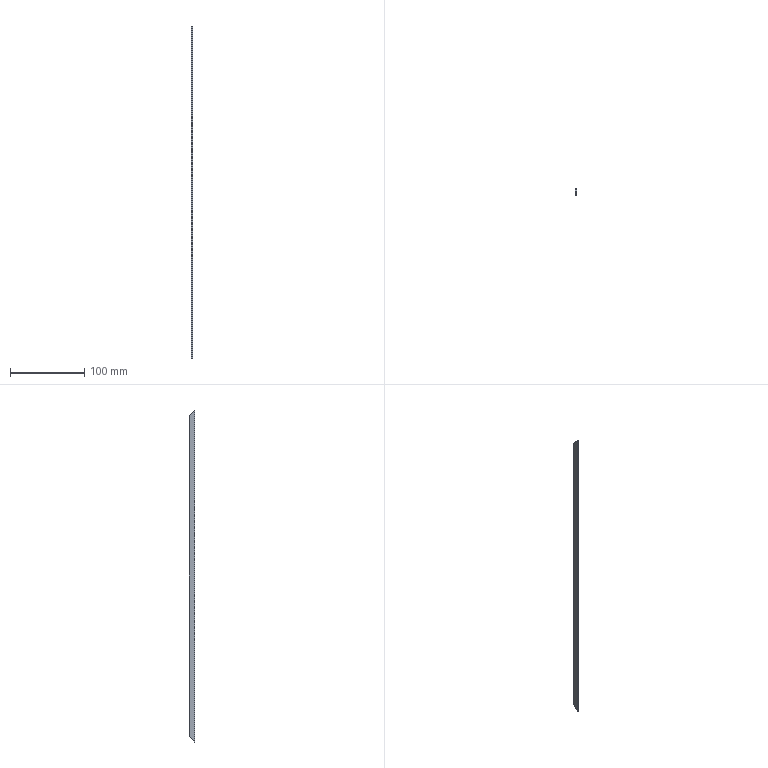Part | NX | features BREP 1 | 1 solid | 6 faces | box 1.5 x 8 x 447.9 mm | volume 5279 mm3 | plane 6
STEP:
#1=CARTESIAN_POINT('',(0.,8.,215.95));
#2=VERTEX_POINT('',#1);
#3=CARTESIAN_POINT('',(0.,8.,-215.95));
#4=VERTEX_POINT('',#3);
#5=CARTESIAN_POINT('',(0.,8.,223.95));
#6=DIRECTION('',(0.,0.,-1.));
#7=VECTOR('',#6,1000.);
#8=LINE('',#5,#7);
#9=EDGE_CURVE('',#2,#4,#8,.T.);
#10=ORIENTED_EDGE('',*,*,#9,.T.);
#11=CARTESIAN_POINT('',(0.,0.,-223.95));
#12=VERTEX_POINT('',#11);
#13=CARTESIAN_POINT('',(0.,8.,-215.95));
#14=DIRECTION('',(0.,-0.7071,-0.7071));
#15=VECTOR('',#14,1000.);
#16=LINE('',#13,#15);
#17=EDGE_CURVE('',#4,#12,#16,.T.);
#18=ORIENTED_EDGE('',*,*,#17,.T.);
#19=CARTESIAN_POINT('',(0.,0.,223.95));
#20=VERTEX_POINT('',#19);
#21=CARTESIAN_POINT('',(0.,0.,223.95));
#22=DIRECTION('',(0.,0.,-1.));
#23=VECTOR('',#22,1000.);
#24=LINE('',#21,#23);
#25=EDGE_CURVE('',#20,#12,#24,.T.);
#26=ORIENTED_EDGE('',*,*,#25,.F.);
#27=CARTESIAN_POINT('',(0.,0.,223.95));
#28=DIRECTION('',(0.,0.7071,-0.7071));
#29=VECTOR('',#28,1000.);
#30=LINE('',#27,#29);
#31=EDGE_CURVE('',#20,#2,#30,.T.);
#32=ORIENTED_EDGE('',*,*,#31,.T.);
#33=EDGE_LOOP('',(#10,#18,#26,#32));
#34=FACE_BOUND('',#33,.T.);
#35=CARTESIAN_POINT('',(0.,0.,223.95));
#36=DIRECTION('',(1.,0.,0.));
#37=DIRECTION('',(0.,1.,0.));
#38=AXIS2_PLACEMENT_3D('',#35,#36,#37);
#39=PLANE('',#38);
#40=ADVANCED_FACE('',(#34),#39,.F.);
#41=CARTESIAN_POINT('',(1.5,0.,-223.95));
#42=VERTEX_POINT('',#41);
#43=CARTESIAN_POINT('',(0.,0.,-223.95));
#44=DIRECTION('',(1.,0.,0.));
#45=VECTOR('',#44,1000.);
#46=LINE('',#43,#45);
#47=EDGE_CURVE('',#12,#42,#46,.T.);
#48=ORIENTED_EDGE('',*,*,#47,.T.);
#49=CARTESIAN_POINT('',(1.5,0.,223.95));
#50=VERTEX_POINT('',#49);
#51=CARTESIAN_POINT('',(1.5,0.,223.95));
#52=DIRECTION('',(0.,0.,-1.));
#53=VECTOR('',#52,1000.);
#54=LINE('',#51,#53);
#55=EDGE_CURVE('',#50,#42,#54,.T.);
#56=ORIENTED_EDGE('',*,*,#55,.F.);
#57=CARTESIAN_POINT('',(0.,0.,223.95));
#58=DIRECTION('',(1.,0.,0.));
#59=VECTOR('',#58,1000.);
#60=LINE('',#57,#59);
#61=EDGE_CURVE('',#20,#50,#60,.T.);
#62=ORIENTED_EDGE('',*,*,#61,.F.);
#63=ORIENTED_EDGE('',*,*,#25,.T.);
#64=EDGE_LOOP('',(#48,#56,#62,#63));
#65=FACE_BOUND('',#64,.T.);
#66=CARTESIAN_POINT('',(0.,0.,223.95));
#67=DIRECTION('',(0.,1.,0.));
#68=DIRECTION('',(1.,0.,0.));
#69=AXIS2_PLACEMENT_3D('',#66,#67,#68);
#70=PLANE('',#69);
#71=ADVANCED_FACE('',(#65),#70,.F.);
#72=ORIENTED_EDGE('',*,*,#55,.T.);
#73=CARTESIAN_POINT('',(1.5,8.,-215.95));
#74=VERTEX_POINT('',#73);
#75=CARTESIAN_POINT('',(1.5,8.,-215.95));
#76=DIRECTION('',(0.,0.7071,0.7071));
#77=VECTOR('',#76,1000.);
#78=LINE('',#75,#77);
#79=EDGE_CURVE('',#42,#74,#78,.T.);
#80=ORIENTED_EDGE('',*,*,#79,.T.);
#81=CARTESIAN_POINT('',(1.5,8.,215.95));
#82=VERTEX_POINT('',#81);
#83=CARTESIAN_POINT('',(1.5,8.,223.95));
#84=DIRECTION('',(0.,0.,-1.));
#85=VECTOR('',#84,1000.);
#86=LINE('',#83,#85);
#87=EDGE_CURVE('',#82,#74,#86,.T.);
#88=ORIENTED_EDGE('',*,*,#87,.F.);
#89=CARTESIAN_POINT('',(1.5,0.,223.95));
#90=DIRECTION('',(0.,-0.7071,0.7071));
#91=VECTOR('',#90,1000.);
#92=LINE('',#89,#91);
#93=EDGE_CURVE('',#82,#50,#92,.T.);
#94=ORIENTED_EDGE('',*,*,#93,.T.);
#95=EDGE_LOOP('',(#72,#80,#88,#94));
#96=FACE_BOUND('',#95,.T.);
#97=CARTESIAN_POINT('',(1.5,0.,223.95));
#98=DIRECTION('',(-1.,0.,0.));
#99=DIRECTION('',(0.,0.,1.));
#100=AXIS2_PLACEMENT_3D('',#97,#98,#99);
#101=PLANE('',#100);
#102=ADVANCED_FACE('',(#96),#101,.F.);
#103=ORIENTED_EDGE('',*,*,#87,.T.);
#104=CARTESIAN_POINT('',(0.,8.,-215.95));
#105=DIRECTION('',(-1.,0.,0.));
#106=VECTOR('',#105,1000.);
#107=LINE('',#104,#106);
#108=EDGE_CURVE('',#74,#4,#107,.T.);
#109=ORIENTED_EDGE('',*,*,#108,.T.);
#110=ORIENTED_EDGE('',*,*,#9,.F.);
#111=CARTESIAN_POINT('',(0.,8.,215.95));
#112=DIRECTION('',(1.,0.,0.));
#113=VECTOR('',#112,1000.);
#114=LINE('',#111,#113);
#115=EDGE_CURVE('',#2,#82,#114,.T.);
#116=ORIENTED_EDGE('',*,*,#115,.T.);
#117=EDGE_LOOP('',(#103,#109,#110,#116));
#118=FACE_BOUND('',#117,.T.);
#119=CARTESIAN_POINT('',(0.,8.,223.95));
#120=DIRECTION('',(0.,-1.,0.));
#121=DIRECTION('',(0.,0.,-1.));
#122=AXIS2_PLACEMENT_3D('',#119,#120,#121);
#123=PLANE('',#122);
#124=ADVANCED_FACE('',(#118),#123,.F.);
#125=ORIENTED_EDGE('',*,*,#79,.F.);
#126=ORIENTED_EDGE('',*,*,#47,.F.);
#127=ORIENTED_EDGE('',*,*,#17,.F.);
#128=ORIENTED_EDGE('',*,*,#108,.F.);
#129=EDGE_LOOP('',(#125,#126,#127,#128));
#130=FACE_BOUND('',#129,.T.);
#131=CARTESIAN_POINT('',(0.,8.,-215.95));
#132=DIRECTION('',(0.,0.7071,-0.7071));
#133=DIRECTION('',(-1.,0.,0.));
#134=AXIS2_PLACEMENT_3D('',#131,#132,#133);
#135=PLANE('',#134);
#136=ADVANCED_FACE('',(#130),#135,.T.);
#137=ORIENTED_EDGE('',*,*,#93,.F.);
#138=ORIENTED_EDGE('',*,*,#115,.F.);
#139=ORIENTED_EDGE('',*,*,#31,.F.);
#140=ORIENTED_EDGE('',*,*,#61,.T.);
#141=EDGE_LOOP('',(#137,#138,#139,#140));
#142=FACE_BOUND('',#141,.T.);
#143=CARTESIAN_POINT('',(0.,0.,223.95));
#144=DIRECTION('',(0.,-0.7071,-0.7071));
#145=DIRECTION('',(0.,-0.7071,0.7071));
#146=AXIS2_PLACEMENT_3D('',#143,#144,#145);
#147=PLANE('',#146);
#148=ADVANCED_FACE('',(#142),#147,.F.);
#149=CLOSED_SHELL('',(#40,#71,#102,#124,#136,#148));
#150=MANIFOLD_SOLID_BREP('',#149);
#151=(LENGTH_UNIT()NAMED_UNIT(*)SI_UNIT(.MILLI.,.METRE.));
#152=UNCERTAINTY_MEASURE_WITH_UNIT(LENGTH_MEASURE(0.00001),#151,'','');
#153=(NAMED_UNIT(*)PLANE_ANGLE_UNIT()SI_UNIT($,.RADIAN.));
#154=(NAMED_UNIT(*)SI_UNIT($,.STERADIAN.)SOLID_ANGLE_UNIT());
#155=(GEOMETRIC_REPRESENTATION_CONTEXT(3)GLOBAL_UNCERTAINTY_ASSIGNED_CONTEXT((#152))GLOBAL_UNIT_ASSIGNED_CONTEXT((#151,#153,#154))REPRESENTATION_CONTEXT('',''));
#156=ADVANCED_BREP_SHAPE_REPRESENTATION('',(#150),#155);